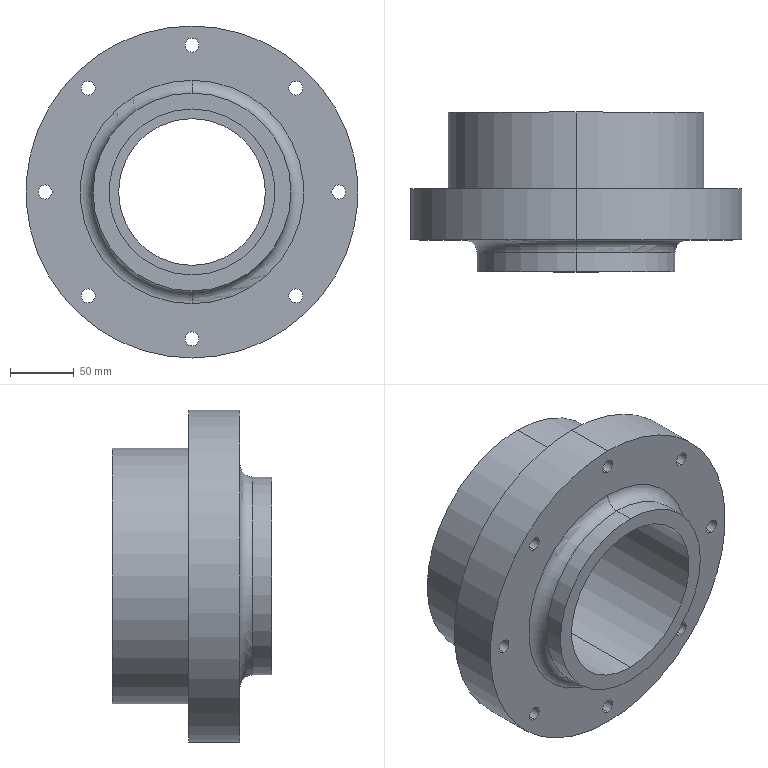Part | SolidWorks | features ICE 3, Revolution 1 | 1 solid | 81 faces | box 260 x 125 x 260 mm | volume 2840283 mm3 | cylinder 58 | plane 21 | torus 2 | commonest cylinder face diameters 10 x16 11 x16 22 x16 115 x2 130 x2 155 x2